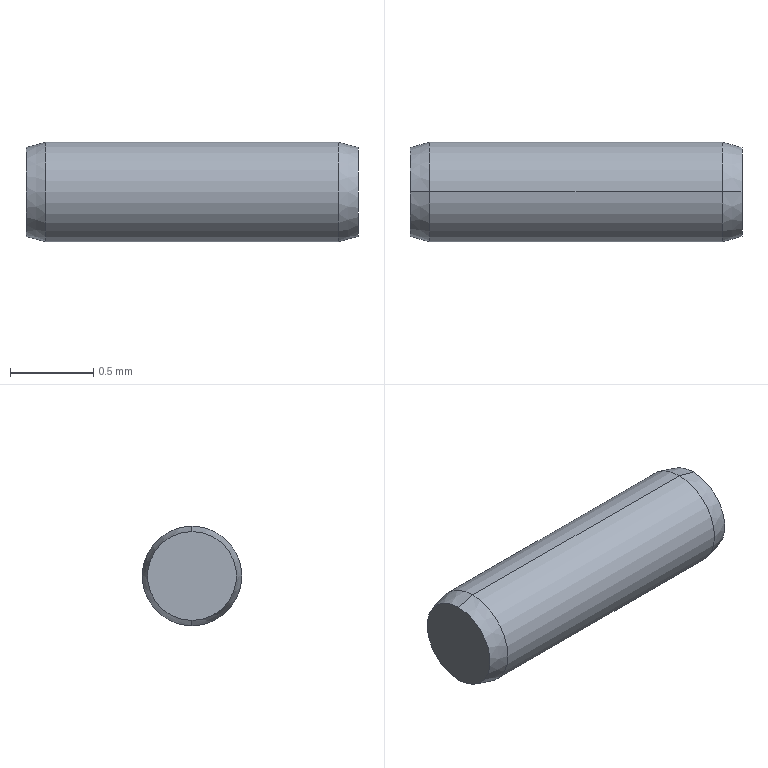Part | SolidWorks | features Revolution 1 | 1 solid | 8 faces | box 2 x 0.6 x 0.6 mm | volume 0.5585 mm3 | cone 4 | cylinder 2 | plane 2 | commonest cylinder face diameters 0.6 x2
STEP:
#1=CARTESIAN_POINT('',(0.,0.,0.2678));
#2=VERTEX_POINT('',#1);
#3=CARTESIAN_POINT('',(0.,0.,-0.2678));
#4=VERTEX_POINT('',#3);
#5=CARTESIAN_POINT('',(0.,0.,0.));
#6=DIRECTION('',(-1.,0.,0.));
#7=DIRECTION('',(0.,0.,1.));
#8=AXIS2_PLACEMENT_3D('',#5,#6,#7);
#9=CIRCLE('',#8,0.2678);
#10=EDGE_CURVE('',#2,#4,#9,.T.);
#11=ORIENTED_EDGE('',*,*,#10,.F.);
#12=CARTESIAN_POINT('',(0.12,0.,0.3));
#13=VERTEX_POINT('',#12);
#14=CARTESIAN_POINT('',(0.12,0.,0.3));
#15=DIRECTION('',(0.9659,0.,0.2588));
#16=VECTOR('',#15,1000.);
#17=LINE('',#14,#16);
#18=EDGE_CURVE('',#2,#13,#17,.T.);
#19=ORIENTED_EDGE('',*,*,#18,.T.);
#20=CARTESIAN_POINT('',(0.12,0.,-0.3));
#21=VERTEX_POINT('',#20);
#22=CARTESIAN_POINT('',(0.12,0.,0.));
#23=DIRECTION('',(-1.,0.,0.));
#24=DIRECTION('',(0.,0.,1.));
#25=AXIS2_PLACEMENT_3D('',#22,#23,#24);
#26=CIRCLE('',#25,0.3);
#27=EDGE_CURVE('',#13,#21,#26,.T.);
#28=ORIENTED_EDGE('',*,*,#27,.T.);
#29=CARTESIAN_POINT('',(0.12,0.,-0.3));
#30=DIRECTION('',(0.9659,0.,-0.2588));
#31=VECTOR('',#30,1000.);
#32=LINE('',#29,#31);
#33=EDGE_CURVE('',#4,#21,#32,.T.);
#34=ORIENTED_EDGE('',*,*,#33,.F.);
#35=EDGE_LOOP('',(#11,#19,#28,#34));
#36=FACE_OUTER_BOUND('',#35,.T.);
#37=CARTESIAN_POINT('',(0.12,0.,0.));
#38=DIRECTION('',(1.,0.,0.));
#39=DIRECTION('',(0.,0.,-1.));
#40=AXIS2_PLACEMENT_3D('',#37,#38,#39);
#41=CONICAL_SURFACE('',#40,0.3,0.2618);
#42=ADVANCED_FACE('',(#36),#41,.T.);
#43=CARTESIAN_POINT('',(1.88,0.,0.3));
#44=VERTEX_POINT('',#43);
#45=CARTESIAN_POINT('',(1.88,0.,-0.3));
#46=VERTEX_POINT('',#45);
#47=CARTESIAN_POINT('',(1.88,0.,0.));
#48=DIRECTION('',(-1.,0.,0.));
#49=DIRECTION('',(0.,0.,1.));
#50=AXIS2_PLACEMENT_3D('',#47,#48,#49);
#51=CIRCLE('',#50,0.3);
#52=EDGE_CURVE('',#44,#46,#51,.T.);
#53=ORIENTED_EDGE('',*,*,#52,.T.);
#54=CARTESIAN_POINT('',(-1.656,0.,-0.3));
#55=DIRECTION('',(-1.,0.,0.));
#56=VECTOR('',#55,1000.);
#57=LINE('',#54,#56);
#58=EDGE_CURVE('',#46,#21,#57,.T.);
#59=ORIENTED_EDGE('',*,*,#58,.T.);
#60=ORIENTED_EDGE('',*,*,#27,.F.);
#61=CARTESIAN_POINT('',(-1.656,0.,0.3));
#62=DIRECTION('',(-1.,0.,0.));
#63=VECTOR('',#62,1000.);
#64=LINE('',#61,#63);
#65=EDGE_CURVE('',#44,#13,#64,.T.);
#66=ORIENTED_EDGE('',*,*,#65,.F.);
#67=EDGE_LOOP('',(#53,#59,#60,#66));
#68=FACE_OUTER_BOUND('',#67,.T.);
#69=CARTESIAN_POINT('',(-1.656,0.,0.));
#70=DIRECTION('',(-1.,0.,0.));
#71=DIRECTION('',(0.,0.,1.));
#72=AXIS2_PLACEMENT_3D('',#69,#70,#71);
#73=CYLINDRICAL_SURFACE('',#72,0.3);
#74=ADVANCED_FACE('',(#68),#73,.T.);
#75=CARTESIAN_POINT('',(2.,0.,0.2678));
#76=VERTEX_POINT('',#75);
#77=CARTESIAN_POINT('',(2.,0.,-0.2678));
#78=VERTEX_POINT('',#77);
#79=CARTESIAN_POINT('',(2.,0.,0.));
#80=DIRECTION('',(-1.,0.,0.));
#81=DIRECTION('',(0.,0.,1.));
#82=AXIS2_PLACEMENT_3D('',#79,#80,#81);
#83=CIRCLE('',#82,0.2678);
#84=EDGE_CURVE('',#76,#78,#83,.T.);
#85=ORIENTED_EDGE('',*,*,#84,.T.);
#86=CARTESIAN_POINT('',(2.,0.,-0.2678));
#87=DIRECTION('',(-0.9659,0.,-0.2588));
#88=VECTOR('',#87,1000.);
#89=LINE('',#86,#88);
#90=EDGE_CURVE('',#78,#46,#89,.T.);
#91=ORIENTED_EDGE('',*,*,#90,.T.);
#92=ORIENTED_EDGE('',*,*,#52,.F.);
#93=CARTESIAN_POINT('',(2.,0.,0.2678));
#94=DIRECTION('',(-0.9659,0.,0.2588));
#95=VECTOR('',#94,1000.);
#96=LINE('',#93,#95);
#97=EDGE_CURVE('',#76,#44,#96,.T.);
#98=ORIENTED_EDGE('',*,*,#97,.F.);
#99=EDGE_LOOP('',(#85,#91,#92,#98));
#100=FACE_OUTER_BOUND('',#99,.T.);
#101=CARTESIAN_POINT('',(2.,0.,0.));
#102=DIRECTION('',(-1.,0.,0.));
#103=DIRECTION('',(0.,0.,1.));
#104=AXIS2_PLACEMENT_3D('',#101,#102,#103);
#105=CONICAL_SURFACE('',#104,0.2678,0.2618);
#106=ADVANCED_FACE('',(#100),#105,.T.);
#107=CARTESIAN_POINT('',(0.,0.,0.));
#108=DIRECTION('',(-1.,0.,0.));
#109=DIRECTION('',(0.,0.,1.));
#110=AXIS2_PLACEMENT_3D('',#107,#108,#109);
#111=CIRCLE('',#110,0.2678);
#112=EDGE_CURVE('',#4,#2,#111,.T.);
#113=ORIENTED_EDGE('',*,*,#112,.T.);
#114=ORIENTED_EDGE('',*,*,#10,.T.);
#115=EDGE_LOOP('',(#113,#114));
#116=FACE_OUTER_BOUND('',#115,.T.);
#117=CARTESIAN_POINT('',(0.,0.2678,0.));
#118=DIRECTION('',(1.,0.,0.));
#119=DIRECTION('',(0.,0.,-1.));
#120=AXIS2_PLACEMENT_3D('',#117,#118,#119);
#121=PLANE('',#120);
#122=ADVANCED_FACE('',(#116),#121,.F.);
#123=ORIENTED_EDGE('',*,*,#84,.F.);
#124=CARTESIAN_POINT('',(2.,0.,0.));
#125=DIRECTION('',(-1.,0.,0.));
#126=DIRECTION('',(0.,0.,1.));
#127=AXIS2_PLACEMENT_3D('',#124,#125,#126);
#128=CIRCLE('',#127,0.2678);
#129=EDGE_CURVE('',#78,#76,#128,.T.);
#130=ORIENTED_EDGE('',*,*,#129,.F.);
#131=EDGE_LOOP('',(#123,#130));
#132=FACE_OUTER_BOUND('',#131,.T.);
#133=CARTESIAN_POINT('',(2.,0.,0.));
#134=DIRECTION('',(-1.,0.,0.));
#135=DIRECTION('',(0.,0.,1.));
#136=AXIS2_PLACEMENT_3D('',#133,#134,#135);
#137=PLANE('',#136);
#138=ADVANCED_FACE('',(#132),#137,.F.);
#139=ORIENTED_EDGE('',*,*,#90,.F.);
#140=ORIENTED_EDGE('',*,*,#129,.T.);
#141=ORIENTED_EDGE('',*,*,#97,.T.);
#142=CARTESIAN_POINT('',(1.88,0.,0.));
#143=DIRECTION('',(-1.,0.,0.));
#144=DIRECTION('',(0.,0.,1.));
#145=AXIS2_PLACEMENT_3D('',#142,#143,#144);
#146=CIRCLE('',#145,0.3);
#147=EDGE_CURVE('',#46,#44,#146,.T.);
#148=ORIENTED_EDGE('',*,*,#147,.F.);
#149=EDGE_LOOP('',(#139,#140,#141,#148));
#150=FACE_OUTER_BOUND('',#149,.T.);
#151=CARTESIAN_POINT('',(2.,0.,0.));
#152=DIRECTION('',(-1.,0.,0.));
#153=DIRECTION('',(0.,0.,1.));
#154=AXIS2_PLACEMENT_3D('',#151,#152,#153);
#155=CONICAL_SURFACE('',#154,0.2678,0.2618);
#156=ADVANCED_FACE('',(#150),#155,.T.);
#157=ORIENTED_EDGE('',*,*,#58,.F.);
#158=ORIENTED_EDGE('',*,*,#147,.T.);
#159=ORIENTED_EDGE('',*,*,#65,.T.);
#160=CARTESIAN_POINT('',(0.12,0.,0.));
#161=DIRECTION('',(-1.,0.,0.));
#162=DIRECTION('',(0.,0.,1.));
#163=AXIS2_PLACEMENT_3D('',#160,#161,#162);
#164=CIRCLE('',#163,0.3);
#165=EDGE_CURVE('',#21,#13,#164,.T.);
#166=ORIENTED_EDGE('',*,*,#165,.F.);
#167=EDGE_LOOP('',(#157,#158,#159,#166));
#168=FACE_OUTER_BOUND('',#167,.T.);
#169=CARTESIAN_POINT('',(-1.656,0.,0.));
#170=DIRECTION('',(-1.,0.,0.));
#171=DIRECTION('',(0.,0.,1.));
#172=AXIS2_PLACEMENT_3D('',#169,#170,#171);
#173=CYLINDRICAL_SURFACE('',#172,0.3);
#174=ADVANCED_FACE('',(#168),#173,.T.);
#175=ORIENTED_EDGE('',*,*,#18,.F.);
#176=ORIENTED_EDGE('',*,*,#112,.F.);
#177=ORIENTED_EDGE('',*,*,#33,.T.);
#178=ORIENTED_EDGE('',*,*,#165,.T.);
#179=EDGE_LOOP('',(#175,#176,#177,#178));
#180=FACE_OUTER_BOUND('',#179,.T.);
#181=CARTESIAN_POINT('',(0.12,0.,0.));
#182=DIRECTION('',(1.,0.,0.));
#183=DIRECTION('',(0.,0.,-1.));
#184=AXIS2_PLACEMENT_3D('',#181,#182,#183);
#185=CONICAL_SURFACE('',#184,0.3,0.2618);
#186=ADVANCED_FACE('',(#180),#185,.T.);
#187=CLOSED_SHELL('',(#42,#74,#106,#122,#138,#156,#174,#186));
#188=MANIFOLD_SOLID_BREP('',#187);
#189=CARTESIAN_POINT('',(0.,0.,0.));
#190=DIRECTION('',(0.,0.,1.));
#191=DIRECTION('',(1.,0.,0.));
#192=AXIS2_PLACEMENT_3D('',#189,#190,#191);
#193=(LENGTH_UNIT()NAMED_UNIT(*)SI_UNIT(.MILLI.,.METRE.));
#194=UNCERTAINTY_MEASURE_WITH_UNIT(LENGTH_MEASURE(0.00001),#193,'','');
#195=(NAMED_UNIT(*)PLANE_ANGLE_UNIT()SI_UNIT($,.RADIAN.));
#196=(NAMED_UNIT(*)SI_UNIT($,.STERADIAN.)SOLID_ANGLE_UNIT());
#197=(GEOMETRIC_REPRESENTATION_CONTEXT(3)GLOBAL_UNCERTAINTY_ASSIGNED_CONTEXT((#194))GLOBAL_UNIT_ASSIGNED_CONTEXT((#193,#195,#196))REPRESENTATION_CONTEXT('',''));
#198=ADVANCED_BREP_SHAPE_REPRESENTATION('',(#188,#192),#197);